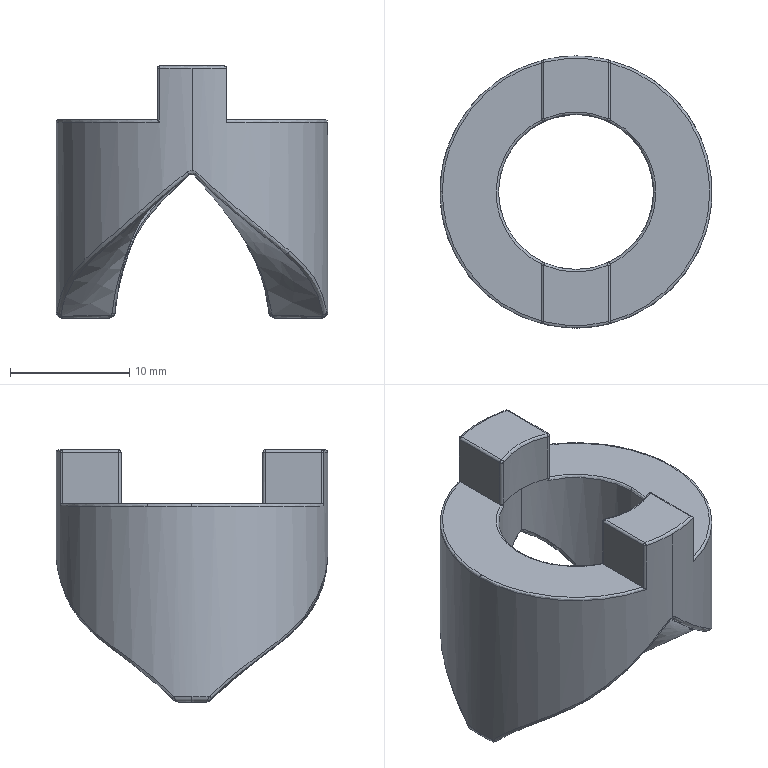Part | STEP file | 101000008265 | 1 solid | 97 faces | box 22.806 x 22.806 x 21.136 mm | volume 3240 mm3 | spline 58 | cylinder 21 | plane 10 | torus 8 | commonest cylinder face diameters 0.4 x15 13 x2 13.002 x2 22.806 x2